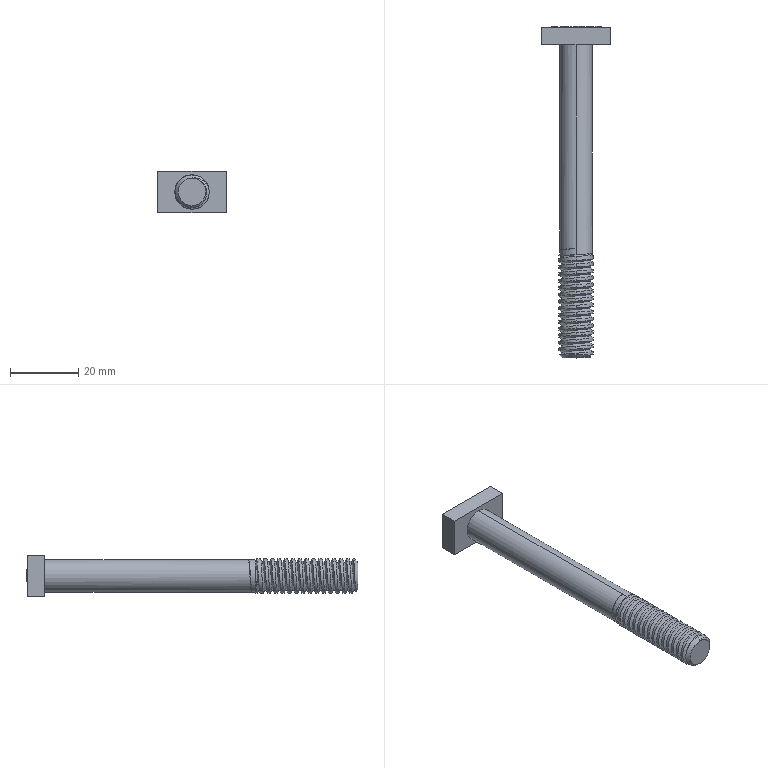Part | SolidWorks | features ICE 2, Chamfer 1, Emboss 1, Extrusion 1, Helix 1, SweepCut 1 | 1 solid | 124 faces | box 20 x 97 x 12 mm | volume 7646 mm3 | plane 60 | cylinder 35 | spline 26 | cone 3 | commonest cylinder face diameters 10 x31 9.5 x4